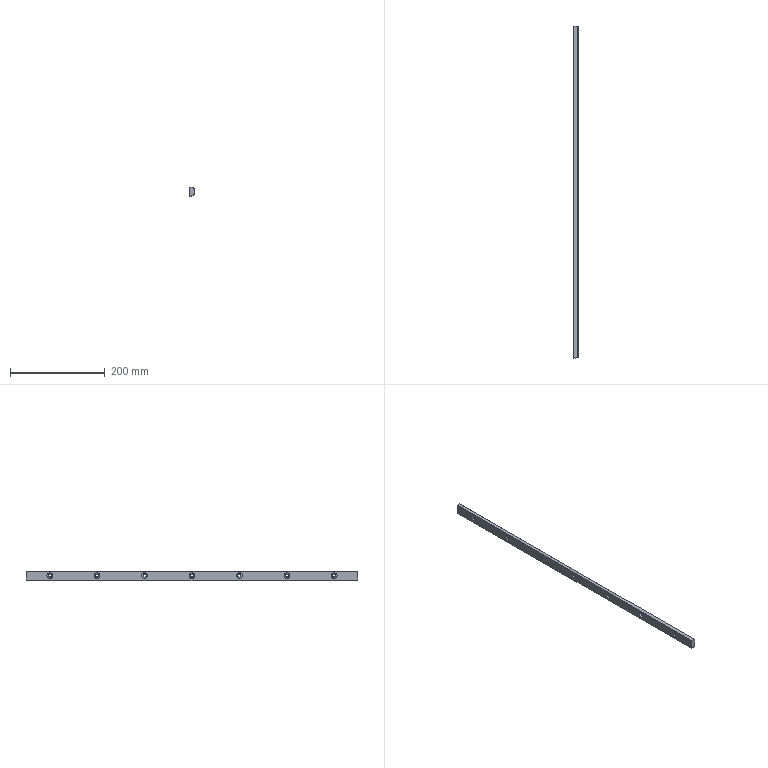Part | STEP file | 06B side guide chain support block | 1 solid | 53 faces | box 9 x 700 x 20.4 mm | volume 110428 mm3 | cylinder 34 | plane 19 | commonest cylinder face diameters 6.5 x14 12 x14 3 x6